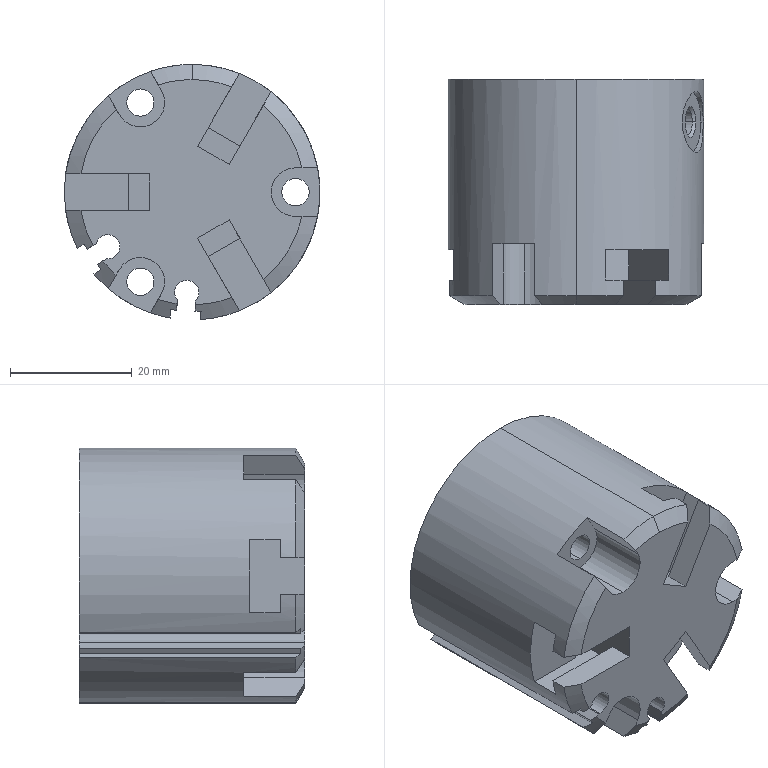Part | SolidWorks | features BaseBody 1 | 1 solid | 128 faces | box 42 x 37 x 41.953 mm | volume 41589 mm3 | plane 60 | cylinder 39 | cone 29 | commonest cylinder face diameters 3.242 x6 4.5 x6 3 x5 4 x5 4.134 x4 8 x4